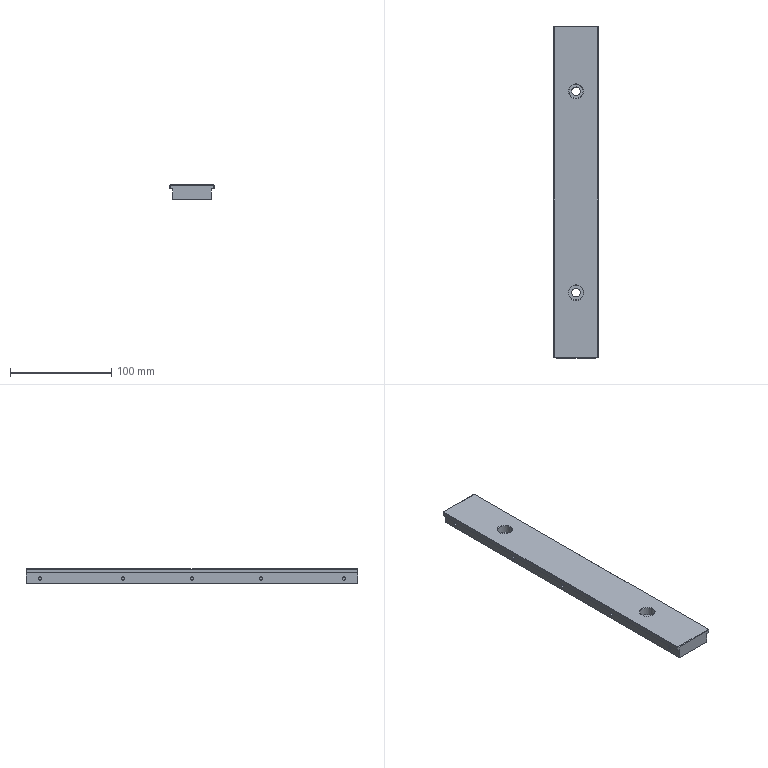Part | 1 solid | 68 faces | box 44 x 328 x 14 mm | volume 177206 mm3 | plane 40 | cylinder 26 | cone 2 | commonest cylinder face diameters 3.2 x10 6.6 x8 16 x4 8.5 x2 14 x1 14.5 x1